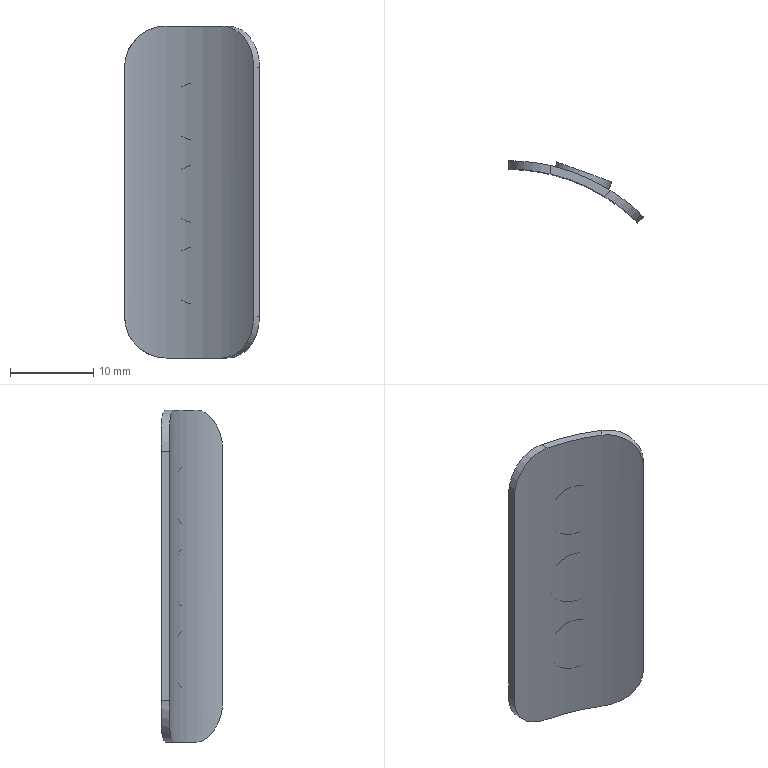Part | NX | features DATUM_CSYS 3, EXTRUDE 2, SKETCH 2, BLEND 1, DATUM_PLANE 1 | 4 solids | 19 faces | box 16.263 x 7.446 x 40 mm | volume 858.511 mm3 | plane 10 | cylinder 9 | commonest cylinder face diameters 10 x4 7 x3 44 x1 46 x1
STEP:
#1=CARTESIAN_POINT('',(5.842,22.882,9.934));
#2=VERTEX_POINT('',#1);
#3=CARTESIAN_POINT('',(9.131,21.685,9.934));
#4=DIRECTION('',(0.342,0.9397,0.));
#5=DIRECTION('',(-0.9397,0.342,0.));
#6=AXIS2_PLACEMENT_3D('',#3,#4,#5);
#7=CIRCLE('',#6,3.5);
#8=EDGE_CURVE('',#2,#2,#7,.T.);
#9=ORIENTED_EDGE('',*,*,#8,.F.);
#10=EDGE_LOOP('',(#9));
#11=FACE_BOUND('',#10,.T.);
#12=CARTESIAN_POINT('',(5.329,21.472,9.934));
#13=VERTEX_POINT('',#12);
#14=CARTESIAN_POINT('',(8.618,20.275,9.934));
#15=DIRECTION('',(0.342,0.9397,0.));
#16=DIRECTION('',(-0.9397,0.342,0.));
#17=AXIS2_PLACEMENT_3D('',#14,#15,#16);
#18=CIRCLE('',#17,3.5);
#19=EDGE_CURVE('',#13,#13,#18,.T.);
#20=ORIENTED_EDGE('',*,*,#19,.T.);
#21=EDGE_LOOP('',(#20));
#22=FACE_BOUND('',#21,.T.);
#23=CARTESIAN_POINT('',(9.131,21.685,9.934));
#24=DIRECTION('',(-0.342,-0.9397,0.));
#25=DIRECTION('',(0.9397,-0.342,0.));
#26=AXIS2_PLACEMENT_3D('',#23,#24,#25);
#27=CYLINDRICAL_SURFACE('',#26,3.5);
#28=ADVANCED_FACE('',(#11,#22),#27,.T.);
#29=ORIENTED_EDGE('',*,*,#8,.T.);
#30=EDGE_LOOP('',(#29));
#31=FACE_BOUND('',#30,.T.);
#32=CARTESIAN_POINT('',(9.131,21.685,9.934));
#33=DIRECTION('',(0.342,0.9397,0.));
#34=DIRECTION('',(-0.9397,0.342,0.));
#35=AXIS2_PLACEMENT_3D('',#32,#33,#34);
#36=PLANE('',#35);
#37=ADVANCED_FACE('',(#31),#36,.T.);
#38=ORIENTED_EDGE('',*,*,#19,.F.);
#39=EDGE_LOOP('',(#38));
#40=FACE_BOUND('',#39,.T.);
#41=CARTESIAN_POINT('',(8.618,20.275,9.934));
#42=DIRECTION('',(0.342,0.9397,0.));
#43=DIRECTION('',(-0.9397,0.342,0.));
#44=AXIS2_PLACEMENT_3D('',#41,#42,#43);
#45=PLANE('',#44);
#46=ADVANCED_FACE('',(#40),#45,.F.);
#47=CLOSED_SHELL('',(#28,#37,#46));
#48=MANIFOLD_SOLID_BREP('',#47);
#49=CARTESIAN_POINT('',(5.842,22.882,29.7));
#50=VERTEX_POINT('',#49);
#51=CARTESIAN_POINT('',(9.131,21.685,29.7));
#52=DIRECTION('',(0.342,0.9397,0.));
#53=DIRECTION('',(-0.9397,0.342,0.));
#54=AXIS2_PLACEMENT_3D('',#51,#52,#53);
#55=CIRCLE('',#54,3.5);
#56=EDGE_CURVE('',#50,#50,#55,.T.);
#57=ORIENTED_EDGE('',*,*,#56,.F.);
#58=EDGE_LOOP('',(#57));
#59=FACE_BOUND('',#58,.T.);
#60=CARTESIAN_POINT('',(5.329,21.472,29.7));
#61=VERTEX_POINT('',#60);
#62=CARTESIAN_POINT('',(8.618,20.275,29.7));
#63=DIRECTION('',(0.342,0.9397,0.));
#64=DIRECTION('',(-0.9397,0.342,0.));
#65=AXIS2_PLACEMENT_3D('',#62,#63,#64);
#66=CIRCLE('',#65,3.5);
#67=EDGE_CURVE('',#61,#61,#66,.T.);
#68=ORIENTED_EDGE('',*,*,#67,.T.);
#69=EDGE_LOOP('',(#68));
#70=FACE_BOUND('',#69,.T.);
#71=CARTESIAN_POINT('',(9.131,21.685,29.7));
#72=DIRECTION('',(-0.342,-0.9397,0.));
#73=DIRECTION('',(0.9397,-0.342,0.));
#74=AXIS2_PLACEMENT_3D('',#71,#72,#73);
#75=CYLINDRICAL_SURFACE('',#74,3.5);
#76=ADVANCED_FACE('',(#59,#70),#75,.T.);
#77=ORIENTED_EDGE('',*,*,#56,.T.);
#78=EDGE_LOOP('',(#77));
#79=FACE_BOUND('',#78,.T.);
#80=CARTESIAN_POINT('',(9.131,21.685,29.7));
#81=DIRECTION('',(0.342,0.9397,0.));
#82=DIRECTION('',(-0.9397,0.342,0.));
#83=AXIS2_PLACEMENT_3D('',#80,#81,#82);
#84=PLANE('',#83);
#85=ADVANCED_FACE('',(#79),#84,.T.);
#86=ORIENTED_EDGE('',*,*,#67,.F.);
#87=EDGE_LOOP('',(#86));
#88=FACE_BOUND('',#87,.T.);
#89=CARTESIAN_POINT('',(8.618,20.275,29.7));
#90=DIRECTION('',(0.342,0.9397,0.));
#91=DIRECTION('',(-0.9397,0.342,0.));
#92=AXIS2_PLACEMENT_3D('',#89,#90,#91);
#93=PLANE('',#92);
#94=ADVANCED_FACE('',(#88),#93,.F.);
#95=CLOSED_SHELL('',(#76,#85,#94));
#96=MANIFOLD_SOLID_BREP('',#95);
#97=CARTESIAN_POINT('',(0.,23.,35.));
#98=VERTEX_POINT('',#97);
#99=CARTESIAN_POINT('',(0.,23.,5.));
#100=VERTEX_POINT('',#99);
#101=CARTESIAN_POINT('',(0.,23.,40.));
#102=DIRECTION('',(0.,0.,-1.));
#103=VECTOR('',#102,1000.);
#104=LINE('',#101,#103);
#105=EDGE_CURVE('',#98,#100,#104,.T.);
#106=ORIENTED_EDGE('',*,*,#105,.T.);
#107=CARTESIAN_POINT('',(0.,22.,5.));
#108=VERTEX_POINT('',#107);
#109=CARTESIAN_POINT('',(0.,22.,5.));
#110=DIRECTION('',(0.,1.,0.));
#111=VECTOR('',#110,1000.);
#112=LINE('',#109,#111);
#113=EDGE_CURVE('',#100,#108,#112,.F.);
#114=ORIENTED_EDGE('',*,*,#113,.T.);
#115=CARTESIAN_POINT('',(0.,22.,35.));
#116=VERTEX_POINT('',#115);
#117=CARTESIAN_POINT('',(0.,22.,40.));
#118=DIRECTION('',(0.,0.,-1.));
#119=VECTOR('',#118,1000.);
#120=LINE('',#117,#119);
#121=EDGE_CURVE('',#116,#108,#120,.T.);
#122=ORIENTED_EDGE('',*,*,#121,.F.);
#123=CARTESIAN_POINT('',(0.,23.,35.));
#124=DIRECTION('',(0.,1.,0.));
#125=VECTOR('',#124,1000.);
#126=LINE('',#123,#125);
#127=EDGE_CURVE('',#116,#98,#126,.T.);
#128=ORIENTED_EDGE('',*,*,#127,.T.);
#129=EDGE_LOOP('',(#106,#114,#122,#128));
#130=FACE_BOUND('',#129,.T.);
#131=CARTESIAN_POINT('',(0.,22.,40.));
#132=DIRECTION('',(-1.,0.,0.));
#133=DIRECTION('',(0.,-1.,0.));
#134=AXIS2_PLACEMENT_3D('',#131,#132,#133);
#135=PLANE('',#134);
#136=ADVANCED_FACE('',(#130),#135,.T.);
#137=CARTESIAN_POINT('',(5.,22.45,0.));
#138=VERTEX_POINT('',#137);
#139=CARTESIAN_POINT('',(12.339,19.41,0.));
#140=VERTEX_POINT('',#139);
#141=CARTESIAN_POINT('',(0.,0.,0.));
#142=DIRECTION('',(0.,0.,-1.));
#143=DIRECTION('',(1.,0.,0.));
#144=AXIS2_PLACEMENT_3D('',#141,#142,#143);
#145=CIRCLE('',#144,23.);
#146=EDGE_CURVE('',#138,#140,#145,.T.);
#147=ORIENTED_EDGE('',*,*,#146,.F.);
#148=CARTESIAN_POINT('',(5.,22.45,0.));
#149=CARTESIAN_POINT('',(3.705,22.738,0.));
#150=CARTESIAN_POINT('',(1.105,23.036,1.064));
#151=CARTESIAN_POINT('',(0.,23.,3.673));
#152=CARTESIAN_POINT('',(0.,23.,5.));
#153=B_SPLINE_CURVE_WITH_KNOTS('',3,(#148,#149,#150,#151,#152),.UNSPECIFIED.,.F.,.F.,(4,1,4),(0.,0.003925,0.007849),.UNSPECIFIED.);
#154=EDGE_CURVE('',#138,#100,#153,.T.);
#155=ORIENTED_EDGE('',*,*,#154,.T.);
#156=ORIENTED_EDGE('',*,*,#105,.F.);
#157=CARTESIAN_POINT('',(5.,22.45,40.));
#158=VERTEX_POINT('',#157);
#159=CARTESIAN_POINT('',(0.,23.,35.));
#160=CARTESIAN_POINT('',(0.,23.,36.327));
#161=CARTESIAN_POINT('',(1.1,23.036,38.931));
#162=CARTESIAN_POINT('',(3.705,22.738,40.));
#163=CARTESIAN_POINT('',(5.,22.45,40.));
#164=B_SPLINE_CURVE_WITH_KNOTS('',3,(#159,#160,#161,#162,#163),.UNSPECIFIED.,.F.,.F.,(4,1,4),(0.,0.003924,0.007849),.UNSPECIFIED.);
#165=EDGE_CURVE('',#98,#158,#164,.T.);
#166=ORIENTED_EDGE('',*,*,#165,.T.);
#167=CARTESIAN_POINT('',(12.339,19.41,40.));
#168=VERTEX_POINT('',#167);
#169=CARTESIAN_POINT('',(0.,0.,40.));
#170=DIRECTION('',(0.,0.,-1.));
#171=DIRECTION('',(1.,0.,0.));
#172=AXIS2_PLACEMENT_3D('',#169,#170,#171);
#173=CIRCLE('',#172,23.);
#174=EDGE_CURVE('',#158,#168,#173,.T.);
#175=ORIENTED_EDGE('',*,*,#174,.T.);
#176=CARTESIAN_POINT('',(16.263,16.263,35.));
#177=VERTEX_POINT('',#176);
#178=CARTESIAN_POINT('',(12.339,19.41,40.));
#179=CARTESIAN_POINT('',(13.459,18.698,40.));
#180=CARTESIAN_POINT('',(15.507,17.07,38.936));
#181=CARTESIAN_POINT('',(16.263,16.263,36.327));
#182=CARTESIAN_POINT('',(16.263,16.263,35.));
#183=B_SPLINE_CURVE_WITH_KNOTS('',3,(#178,#179,#180,#181,#182),.UNSPECIFIED.,.F.,.F.,(4,1,4),(0.,0.003925,0.007849),.UNSPECIFIED.);
#184=EDGE_CURVE('',#168,#177,#183,.T.);
#185=ORIENTED_EDGE('',*,*,#184,.T.);
#186=CARTESIAN_POINT('',(16.263,16.263,5.));
#187=VERTEX_POINT('',#186);
#188=CARTESIAN_POINT('',(16.263,16.263,40.));
#189=DIRECTION('',(0.,0.,-1.));
#190=VECTOR('',#189,1000.);
#191=LINE('',#188,#190);
#192=EDGE_CURVE('',#177,#187,#191,.T.);
#193=ORIENTED_EDGE('',*,*,#192,.T.);
#194=CARTESIAN_POINT('',(16.263,16.263,5.));
#195=CARTESIAN_POINT('',(16.263,16.263,3.673));
#196=CARTESIAN_POINT('',(15.511,17.067,1.069));
#197=CARTESIAN_POINT('',(13.459,18.698,0.));
#198=CARTESIAN_POINT('',(12.339,19.41,0.));
#199=B_SPLINE_CURVE_WITH_KNOTS('',3,(#194,#195,#196,#197,#198),.UNSPECIFIED.,.F.,.F.,(4,1,4),(0.,0.003924,0.007849),.UNSPECIFIED.);
#200=EDGE_CURVE('',#187,#140,#199,.T.);
#201=ORIENTED_EDGE('',*,*,#200,.T.);
#202=EDGE_LOOP('',(#147,#155,#156,#166,#175,#185,#193,#201));
#203=FACE_BOUND('',#202,.T.);
#204=CARTESIAN_POINT('',(0.,0.,40.));
#205=DIRECTION('',(0.,0.,-1.));
#206=DIRECTION('',(-1.,0.,0.));
#207=AXIS2_PLACEMENT_3D('',#204,#205,#206);
#208=CYLINDRICAL_SURFACE('',#207,23.);
#209=ADVANCED_FACE('',(#203),#208,.T.);
#210=CARTESIAN_POINT('',(15.556,15.556,35.));
#211=VERTEX_POINT('',#210);
#212=CARTESIAN_POINT('',(15.556,15.556,5.));
#213=VERTEX_POINT('',#212);
#214=CARTESIAN_POINT('',(15.556,15.556,40.));
#215=DIRECTION('',(0.,0.,-1.));
#216=VECTOR('',#215,1000.);
#217=LINE('',#214,#216);
#218=EDGE_CURVE('',#211,#213,#217,.T.);
#219=ORIENTED_EDGE('',*,*,#218,.T.);
#220=CARTESIAN_POINT('',(16.263,16.263,5.));
#221=DIRECTION('',(-0.7071,-0.7071,0.));
#222=VECTOR('',#221,1000.);
#223=LINE('',#220,#222);
#224=EDGE_CURVE('',#213,#187,#223,.F.);
#225=ORIENTED_EDGE('',*,*,#224,.T.);
#226=ORIENTED_EDGE('',*,*,#192,.F.);
#227=CARTESIAN_POINT('',(15.556,15.556,35.));
#228=DIRECTION('',(-0.7071,-0.7071,0.));
#229=VECTOR('',#228,1000.);
#230=LINE('',#227,#229);
#231=EDGE_CURVE('',#177,#211,#230,.T.);
#232=ORIENTED_EDGE('',*,*,#231,.T.);
#233=EDGE_LOOP('',(#219,#225,#226,#232));
#234=FACE_BOUND('',#233,.T.);
#235=CARTESIAN_POINT('',(16.263,16.263,40.));
#236=DIRECTION('',(0.7071,-0.7071,0.));
#237=DIRECTION('',(0.7071,0.7071,0.));
#238=AXIS2_PLACEMENT_3D('',#235,#236,#237);
#239=PLANE('',#238);
#240=ADVANCED_FACE('',(#234),#239,.T.);
#241=ORIENTED_EDGE('',*,*,#121,.T.);
#242=CARTESIAN_POINT('',(5.,21.424,0.));
#243=VERTEX_POINT('',#242);
#244=CARTESIAN_POINT('',(0.,22.,5.));
#245=CARTESIAN_POINT('',(0.,22.,3.672));
#246=CARTESIAN_POINT('',(1.101,22.038,1.067));
#247=CARTESIAN_POINT('',(3.707,21.726,0.));
#248=CARTESIAN_POINT('',(5.,21.424,0.));
#249=B_SPLINE_CURVE_WITH_KNOTS('',3,(#244,#245,#246,#247,#248),.UNSPECIFIED.,.F.,.F.,(4,1,4),(0.,0.003926,0.007853),.UNSPECIFIED.);
#250=EDGE_CURVE('',#108,#243,#249,.T.);
#251=ORIENTED_EDGE('',*,*,#250,.T.);
#252=CARTESIAN_POINT('',(11.614,18.685,0.));
#253=VERTEX_POINT('',#252);
#254=CARTESIAN_POINT('',(0.,0.,0.));
#255=DIRECTION('',(0.,0.,1.));
#256=DIRECTION('',(1.,0.,0.));
#257=AXIS2_PLACEMENT_3D('',#254,#255,#256);
#258=CIRCLE('',#257,22.);
#259=EDGE_CURVE('',#253,#243,#258,.T.);
#260=ORIENTED_EDGE('',*,*,#259,.F.);
#261=CARTESIAN_POINT('',(11.614,18.685,0.));
#262=CARTESIAN_POINT('',(12.741,17.984,0.));
#263=CARTESIAN_POINT('',(14.8,16.365,1.061));
#264=CARTESIAN_POINT('',(15.556,15.556,3.672));
#265=CARTESIAN_POINT('',(15.556,15.556,5.));
#266=B_SPLINE_CURVE_WITH_KNOTS('',3,(#261,#262,#263,#264,#265),.UNSPECIFIED.,.F.,.F.,(4,1,4),(0.,0.003927,0.007853),.UNSPECIFIED.);
#267=EDGE_CURVE('',#253,#213,#266,.T.);
#268=ORIENTED_EDGE('',*,*,#267,.T.);
#269=ORIENTED_EDGE('',*,*,#218,.F.);
#270=CARTESIAN_POINT('',(11.614,18.685,40.));
#271=VERTEX_POINT('',#270);
#272=CARTESIAN_POINT('',(15.556,15.556,35.));
#273=CARTESIAN_POINT('',(15.556,15.556,36.328));
#274=CARTESIAN_POINT('',(14.804,16.362,38.933));
#275=CARTESIAN_POINT('',(12.741,17.984,40.));
#276=CARTESIAN_POINT('',(11.614,18.685,40.));
#277=B_SPLINE_CURVE_WITH_KNOTS('',3,(#272,#273,#274,#275,#276),.UNSPECIFIED.,.F.,.F.,(4,1,4),(0.,0.003926,0.007853),.UNSPECIFIED.);
#278=EDGE_CURVE('',#211,#271,#277,.T.);
#279=ORIENTED_EDGE('',*,*,#278,.T.);
#280=CARTESIAN_POINT('',(5.,21.424,40.));
#281=VERTEX_POINT('',#280);
#282=CARTESIAN_POINT('',(0.,0.,40.));
#283=DIRECTION('',(0.,0.,1.));
#284=DIRECTION('',(1.,0.,0.));
#285=AXIS2_PLACEMENT_3D('',#282,#283,#284);
#286=CIRCLE('',#285,22.);
#287=EDGE_CURVE('',#271,#281,#286,.T.);
#288=ORIENTED_EDGE('',*,*,#287,.T.);
#289=CARTESIAN_POINT('',(5.,21.424,40.));
#290=CARTESIAN_POINT('',(3.708,21.726,40.));
#291=CARTESIAN_POINT('',(1.107,22.037,38.939));
#292=CARTESIAN_POINT('',(0.,22.,36.328));
#293=CARTESIAN_POINT('',(0.,22.,35.));
#294=B_SPLINE_CURVE_WITH_KNOTS('',3,(#289,#290,#291,#292,#293),.UNSPECIFIED.,.F.,.F.,(4,1,4),(0.,0.003927,0.007853),.UNSPECIFIED.);
#295=EDGE_CURVE('',#281,#116,#294,.T.);
#296=ORIENTED_EDGE('',*,*,#295,.T.);
#297=EDGE_LOOP('',(#241,#251,#260,#268,#269,#279,#288,#296));
#298=FACE_BOUND('',#297,.T.);
#299=CARTESIAN_POINT('',(0.,0.,40.));
#300=DIRECTION('',(0.,0.,-1.));
#301=DIRECTION('',(-1.,0.,0.));
#302=AXIS2_PLACEMENT_3D('',#299,#300,#301);
#303=CYLINDRICAL_SURFACE('',#302,22.);
#304=ADVANCED_FACE('',(#298),#303,.F.);
#305=ORIENTED_EDGE('',*,*,#287,.F.);
#306=CARTESIAN_POINT('',(12.728,19.799,40.));
#307=DIRECTION('',(-0.7071,-0.7071,0.));
#308=VECTOR('',#307,1000.);
#309=LINE('',#306,#308);
#310=EDGE_CURVE('',#271,#168,#309,.F.);
#311=ORIENTED_EDGE('',*,*,#310,.T.);
#312=ORIENTED_EDGE('',*,*,#174,.F.);
#313=CARTESIAN_POINT('',(5.,22.,40.));
#314=DIRECTION('',(0.,1.,0.));
#315=VECTOR('',#314,1000.);
#316=LINE('',#313,#315);
#317=EDGE_CURVE('',#158,#281,#316,.F.);
#318=ORIENTED_EDGE('',*,*,#317,.T.);
#319=EDGE_LOOP('',(#305,#311,#312,#318));
#320=FACE_BOUND('',#319,.T.);
#321=CARTESIAN_POINT('',(0.,0.,40.));
#322=DIRECTION('',(0.,0.,-1.));
#323=DIRECTION('',(-1.,0.,0.));
#324=AXIS2_PLACEMENT_3D('',#321,#322,#323);
#325=PLANE('',#324);
#326=ADVANCED_FACE('',(#320),#325,.F.);
#327=ORIENTED_EDGE('',*,*,#259,.T.);
#328=CARTESIAN_POINT('',(5.,0.,0.));
#329=DIRECTION('',(0.,1.,0.));
#330=VECTOR('',#329,1000.);
#331=LINE('',#328,#330);
#332=EDGE_CURVE('',#243,#138,#331,.T.);
#333=ORIENTED_EDGE('',*,*,#332,.T.);
#334=ORIENTED_EDGE('',*,*,#146,.T.);
#335=CARTESIAN_POINT('',(-3.536,3.536,0.));
#336=DIRECTION('',(-0.7071,-0.7071,0.));
#337=VECTOR('',#336,1000.);
#338=LINE('',#335,#337);
#339=EDGE_CURVE('',#140,#253,#338,.T.);
#340=ORIENTED_EDGE('',*,*,#339,.T.);
#341=EDGE_LOOP('',(#327,#333,#334,#340));
#342=FACE_BOUND('',#341,.T.);
#343=CARTESIAN_POINT('',(0.,0.,0.));
#344=DIRECTION('',(0.,0.,-1.));
#345=DIRECTION('',(-1.,0.,0.));
#346=AXIS2_PLACEMENT_3D('',#343,#344,#345);
#347=PLANE('',#346);
#348=ADVANCED_FACE('',(#342),#347,.T.);
#349=ORIENTED_EDGE('',*,*,#250,.F.);
#350=ORIENTED_EDGE('',*,*,#113,.F.);
#351=ORIENTED_EDGE('',*,*,#154,.F.);
#352=ORIENTED_EDGE('',*,*,#332,.F.);
#353=EDGE_LOOP('',(#349,#350,#351,#352));
#354=FACE_BOUND('',#353,.T.);
#355=CARTESIAN_POINT('',(5.,0.,5.));
#356=DIRECTION('',(0.,1.,0.));
#357=DIRECTION('',(-1.,0.,0.));
#358=AXIS2_PLACEMENT_3D('',#355,#356,#357);
#359=CYLINDRICAL_SURFACE('',#358,5.);
#360=ADVANCED_FACE('',(#354),#359,.T.);
#361=ORIENTED_EDGE('',*,*,#200,.F.);
#362=ORIENTED_EDGE('',*,*,#224,.F.);
#363=ORIENTED_EDGE('',*,*,#267,.F.);
#364=ORIENTED_EDGE('',*,*,#339,.F.);
#365=EDGE_LOOP('',(#361,#362,#363,#364));
#366=FACE_BOUND('',#365,.T.);
#367=CARTESIAN_POINT('',(-3.536,3.536,5.));
#368=DIRECTION('',(-0.7071,-0.7071,0.));
#369=DIRECTION('',(0.7071,-0.7071,0.));
#370=AXIS2_PLACEMENT_3D('',#367,#368,#369);
#371=CYLINDRICAL_SURFACE('',#370,5.);
#372=ADVANCED_FACE('',(#366),#371,.T.);
#373=ORIENTED_EDGE('',*,*,#184,.F.);
#374=ORIENTED_EDGE('',*,*,#310,.F.);
#375=ORIENTED_EDGE('',*,*,#278,.F.);
#376=ORIENTED_EDGE('',*,*,#231,.F.);
#377=EDGE_LOOP('',(#373,#374,#375,#376));
#378=FACE_BOUND('',#377,.T.);
#379=CARTESIAN_POINT('',(12.728,19.799,35.));
#380=DIRECTION('',(0.7071,0.7071,0.));
#381=DIRECTION('',(-0.7071,0.7071,0.));
#382=AXIS2_PLACEMENT_3D('',#379,#380,#381);
#383=CYLINDRICAL_SURFACE('',#382,5.);
#384=ADVANCED_FACE('',(#378),#383,.T.);
#385=ORIENTED_EDGE('',*,*,#295,.F.);
#386=ORIENTED_EDGE('',*,*,#317,.F.);
#387=ORIENTED_EDGE('',*,*,#165,.F.);
#388=ORIENTED_EDGE('',*,*,#127,.F.);
#389=EDGE_LOOP('',(#385,#386,#387,#388));
#390=FACE_BOUND('',#389,.T.);
#391=CARTESIAN_POINT('',(5.,22.,35.));
#392=DIRECTION('',(0.,-1.,0.));
#393=DIRECTION('',(1.,0.,0.));
#394=AXIS2_PLACEMENT_3D('',#391,#392,#393);
#395=CYLINDRICAL_SURFACE('',#394,5.);
#396=ADVANCED_FACE('',(#390),#395,.T.);
#397=CLOSED_SHELL('',(#136,#209,#240,#304,#326,#348,#360,#372,#384,#396));
#398=MANIFOLD_SOLID_BREP('',#397);
#399=CARTESIAN_POINT('',(5.842,22.882,19.762));
#400=VERTEX_POINT('',#399);
#401=CARTESIAN_POINT('',(9.131,21.685,19.762));
#402=DIRECTION('',(0.342,0.9397,0.));
#403=DIRECTION('',(-0.9397,0.342,0.));
#404=AXIS2_PLACEMENT_3D('',#401,#402,#403);
#405=CIRCLE('',#404,3.5);
#406=EDGE_CURVE('',#400,#400,#405,.T.);
#407=ORIENTED_EDGE('',*,*,#406,.F.);
#408=EDGE_LOOP('',(#407));
#409=FACE_BOUND('',#408,.T.);
#410=CARTESIAN_POINT('',(5.329,21.472,19.762));
#411=VERTEX_POINT('',#410);
#412=CARTESIAN_POINT('',(8.618,20.275,19.762));
#413=DIRECTION('',(0.342,0.9397,0.));
#414=DIRECTION('',(-0.9397,0.342,0.));
#415=AXIS2_PLACEMENT_3D('',#412,#413,#414);
#416=CIRCLE('',#415,3.5);
#417=EDGE_CURVE('',#411,#411,#416,.T.);
#418=ORIENTED_EDGE('',*,*,#417,.T.);
#419=EDGE_LOOP('',(#418));
#420=FACE_BOUND('',#419,.T.);
#421=CARTESIAN_POINT('',(9.131,21.685,19.762));
#422=DIRECTION('',(-0.342,-0.9397,0.));
#423=DIRECTION('',(0.9397,-0.342,0.));
#424=AXIS2_PLACEMENT_3D('',#421,#422,#423);
#425=CYLINDRICAL_SURFACE('',#424,3.5);
#426=ADVANCED_FACE('',(#409,#420),#425,.T.);
#427=ORIENTED_EDGE('',*,*,#406,.T.);
#428=EDGE_LOOP('',(#427));
#429=FACE_BOUND('',#428,.T.);
#430=CARTESIAN_POINT('',(9.131,21.685,19.762));
#431=DIRECTION('',(0.342,0.9397,0.));
#432=DIRECTION('',(-0.9397,0.342,0.));
#433=AXIS2_PLACEMENT_3D('',#430,#431,#432);
#434=PLANE('',#433);
#435=ADVANCED_FACE('',(#429),#434,.T.);
#436=ORIENTED_EDGE('',*,*,#417,.F.);
#437=EDGE_LOOP('',(#436));
#438=FACE_BOUND('',#437,.T.);
#439=CARTESIAN_POINT('',(8.618,20.275,19.762));
#440=DIRECTION('',(0.342,0.9397,0.));
#441=DIRECTION('',(-0.9397,0.342,0.));
#442=AXIS2_PLACEMENT_3D('',#439,#440,#441);
#443=PLANE('',#442);
#444=ADVANCED_FACE('',(#438),#443,.F.);
#445=CLOSED_SHELL('',(#426,#435,#444));
#446=MANIFOLD_SOLID_BREP('',#445);
#447=(LENGTH_UNIT()NAMED_UNIT(*)SI_UNIT(.MILLI.,.METRE.));
#448=UNCERTAINTY_MEASURE_WITH_UNIT(LENGTH_MEASURE(0.0508),#447,'','');
#449=(NAMED_UNIT(*)PLANE_ANGLE_UNIT()SI_UNIT($,.RADIAN.));
#450=(NAMED_UNIT(*)SI_UNIT($,.STERADIAN.)SOLID_ANGLE_UNIT());
#451=(GEOMETRIC_REPRESENTATION_CONTEXT(3)GLOBAL_UNCERTAINTY_ASSIGNED_CONTEXT((#448))GLOBAL_UNIT_ASSIGNED_CONTEXT((#447,#449,#450))REPRESENTATION_CONTEXT('',''));
#452=ADVANCED_BREP_SHAPE_REPRESENTATION('',(#48,#96,#398,#446),#451);